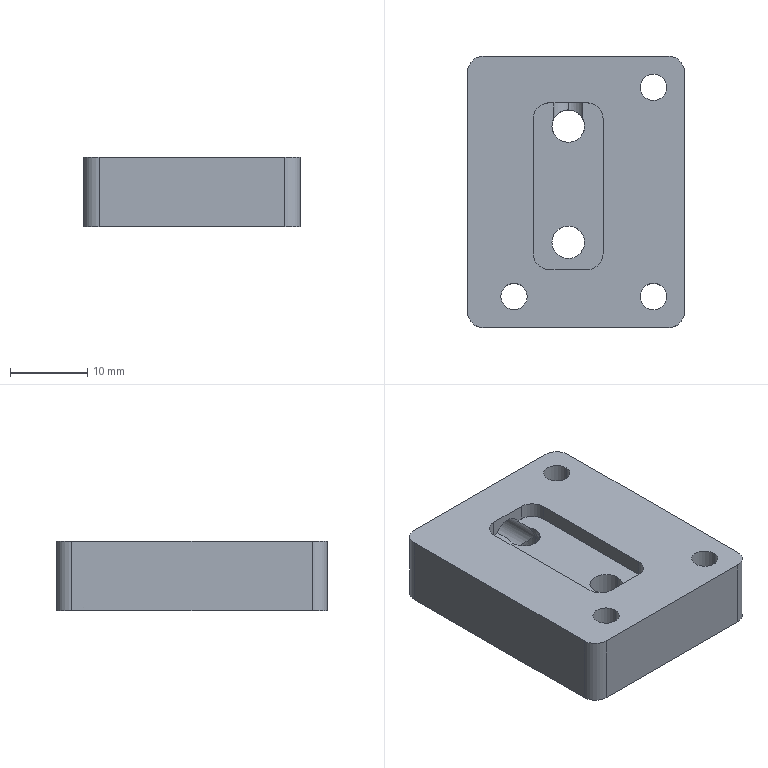Part | STEP file | 11-FG-SB00911 | 1 solid | 49 faces | box 28 x 35 x 9 mm | volume 7627 mm3 | cylinder 31 | plane 14 | cone 4 | commonest cylinder face diameters 4.2 x11 4 x8 3.4 x6 6.5 x6